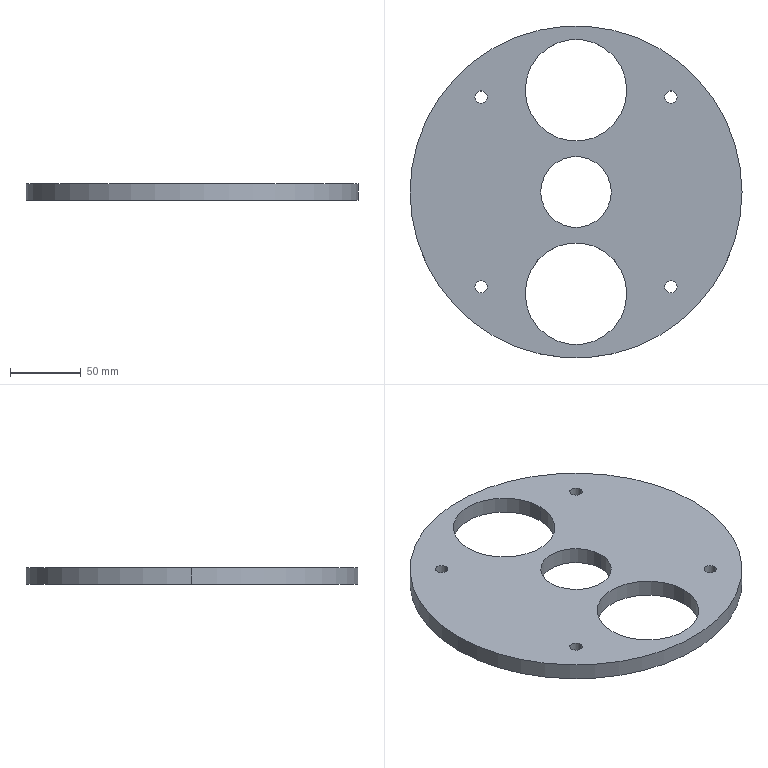Part | STEP file | Sealing disc SGN-2-22 | 1 solid | 30 faces | box 235 x 235 x 12 mm | volume 396002 mm3 | cylinder 22 | cone 6 | plane 2 | commonest cylinder face diameters 8.7 x8 4.2 x6 72 x4 50 x2 235 x2